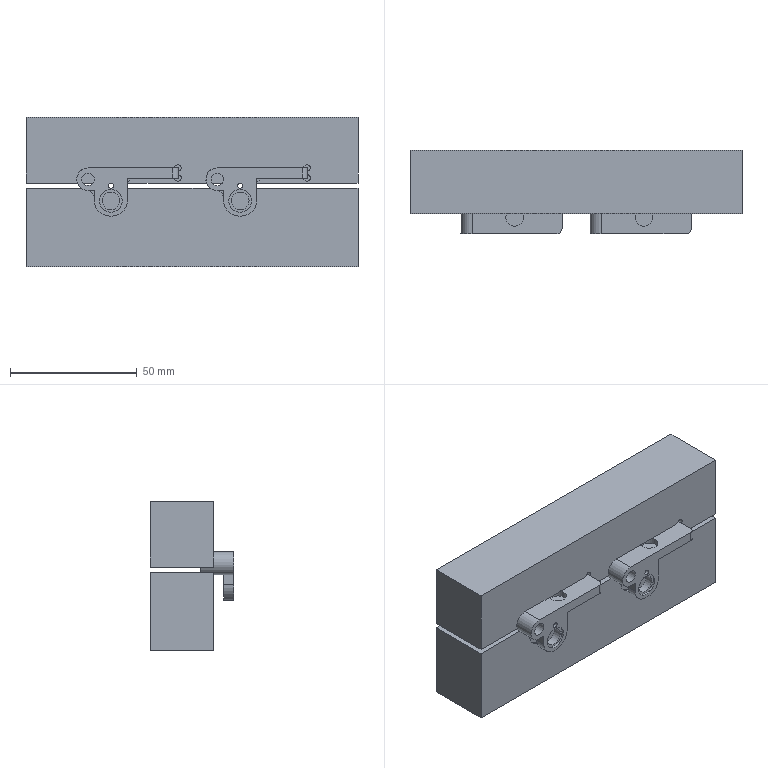CAM job | NX | 3+2 milling, drilling | part box 131 x 33 x 59 mm
Tools:
number,name,description,diameter,corner_radius,flute_length,length,flutes
3,D3,平底铣刀-粗,3.0,0.0,20.0,75.0,2
4,D4,平底铣刀-粗,4.0,0.0,25.0,75.0,2
8,D8,平底铣刀-粗,8.0,0.0,30.0,75.0,2
9,D10,平底铣刀-粗,10.0,0.0,35.0,75.0,2
17,D2-J,平底铣刀-精,2.0,0.0,50.0,75.0,2
11,D4-J,平底铣刀-精,4.0,0.0,50.0,75.0,2
7,D6-J,平底铣刀-精,6.0,0.0,25.0,75.0,2
10,D10-J,平底铣刀-精,10.0,0.0,35.0,75.0,2
1,D80R0.8飞刀,圆鼻刀-粗,80.0,0.8,50.0,75.0,2
2,D6倒角刀,倒角刀,6.0,0.0,3.0,25.0,2
19,M2.5X0.45,丝锥,2.05,0.0,35.0,50.0,2
20,D5铰刀,Drilling Tool,5.0,0.0,75.0,100.0,6
17,ZT2.1,钻头,2.1,0.0,35.0,50.0,2
18,ZT4.9,Drilling Tool,4.9,0.0,35.0,50.0,2
16,ZT6.9,Drilling Tool,6.9,0.0,35.0,50.0,2
Operations:
program,operation,operation_type,tool,method,geometry_group,spindle_rpm,surface_speed,feed_per_tooth,feed_cut,feed_plunge,cut_length_mm,path_length_mm,cut_time_min,machine_time_min
E,BOTTOMWALL-LAYERROUGH-MED_COPY,VolumeBased25DMillingOperation,D3,LAYERROUGH-DEPTHK-STEPG,W-E,8000.0,75.398,0.125,2000.0,100.0,7701.758,7880.728,3.851,3.869
E,ZLEVEL-SMOOTH-CORNERD2-REF6_COPY_2,ZLevelMilling,D2-J,LAYERFINISH-DEPTHK-STEPG,W-E,8000.0,50.264,0.05,800.0,100.0,1220.015,1495.166,1.525,1.552
E,BOTTOMWALL-FINISHFLOOR-MED_COPY_2,VolumeBased25DMillingOperation,D2-J,FINISH-STEPDEPTH-OFF,W-E,7000.0,175.0,0.0536,1500.0,100.0,533.255,631.029,0.3555,0.3653
E,BOTTOMWALL-FINISHFLOOR-MED_COPY_2_COPY,VolumeBased25DMillingOperation,D2-J,FINISH-STEPDEPTH-OFF,W-E,7000.0,175.0,0.0536,1500.0,100.0,244.848,349.977,0.1632,0.1737
E,C0.3CLOSEDCONTOUR-CHAMFER6X45L_COPY_1,PlanarMilling,D6倒角刀,WALLCLIMB_CHAMFER-DEPTH0-STEPG,W-E,7000.0,131.0,0.1071,1500.0,100.0,242.143,477.193,0.1614,0.1849
E,BOTTOMWALL-FINISHSIDE-MED_COPY_1,VolumeBased25DMillingOperation,D2-J,SIDEFINISH-DEPTHK-STEPG,W-E,8000.0,50.264,0.0375,600.0,100.0,148.402,265.878,0.2473,0.2591
E,BOTTOMWALL-FINISHSIDE-MED_COPY_2,VolumeBased25DMillingOperation,D2-J,SIDEFINISH-DEPTHK-STEPG,W-E,8000.0,50.264,0.0375,600.0,100.0,719.738,928.916,1.2,1.22
D,BOTTOMWALL-FINISHSIDE-MED_COPY,VolumeBased25DMillingOperation,D4,SIDEFINISH-DEPTHK-STEPG,W-D,8000.0,100.531,0.125,2000.0,100.0,1801.594,1936.513,0.9008,0.9143
D,BOTTOMWALL-FINISHFLOOR-MED_COPY_1,VolumeBased25DMillingOperation,D4-J,FINISH-STEPDEPTH-OFF,W-D,7000.0,175.0,0.0536,1500.0,100.0,196.489,244.289,0.131,0.1358
D,BOTTOMWALL-FINISHSIDE-MED-SELFLOOR_COPY_1,VolumeBased25DMillingOperation,D4-J,SIDEFINISH-DEPTHK-STEPG,W-D,8000.0,100.528,0.05,800.0,100.0,43.658,96.602,0.0546,0.0599
D,BOTTOMWALL-FINISHSIDE-MED-SELFLOOR_COPY,VolumeBased25DMillingOperation,D4-J,SIDEFINISH-DEPTHK-STEPG,W-D,8000.0,100.528,0.05,800.0,100.0,154.98,232.252,0.1937,0.2015
D,ZLEVEL-SMOOTH-CORNERD2-REF6_COPY_1,ZLevelMilling,D2-J,LAYERFINISH-DEPTHK-STEPG,W-D,8000.0,50.264,0.05,800.0,100.0,411.487,567.042,0.5144,0.5299
C,BOTTOMWALL-HELIXROUGH-SMALL_COPY_1,VolumeBased25DMillingOperation,D4,LAYERROUGH-DEPTHK-STEPG,W-C,8000.0,100.531,0.0375,600.0,100.0,107.628,208.468,0.1794,0.1895
C,C0.3CLOSEDCONTOUR-CHAMFER6X45L_COPY,PlanarMilling,D6倒角刀,WALLCLIMB_CHAMFER-DEPTH0-STEPG,W-C,7000.0,131.0,0.1071,1500.0,100.0,30.826,126.826,0.0206,0.0302
C,BOTTOMWALL-HELIXFINISH-SMALL_COPY_1,VolumeBased25DMillingOperation,D4-J,HELIXFINISH-DEPTHK-STEPG,W-C,8000.0,100.531,0.0312,500.0,100.0,39.572,140.572,0.0791,0.0892
B,DYNAMICROUGHD10_COPY_1,CavityMilling,D10,DYNAMICROUGH-DEPTHK-STEPK,W-B,8000.0,251.32,0.25,4000.0,100.0,4082.757,4178.557,1.021,1.03
B,BOTTOMWALL-FINISHFLOOR-MED_COPY,VolumeBased25DMillingOperation,D10-J,FINISH-STEPDEPTH-OFF,W-B,7000.0,175.0,0.0536,1500.0,100.0,464.965,513.828,0.31,0.3149
B,BOTTOMWALL-HELIXROUGH-SMALL_COPY,VolumeBased25DMillingOperation,D4,LAYERROUGH-DEPTHK-STEPG,W-B,8000.0,100.528,0.125,2000.0,100.0,183.783,432.172,0.0919,0.1167
B,DRILLCHAMFER-DJ10_1,Operation,D6倒角刀,METHOD,W-B,8000.0,150.796,0.0625,1000.0,0.0,11.6,177.288,0.0116,0.0282
B,DRILLCHAMFER_2,Operation,D6倒角刀,METHOD,W-B,8000.0,150.796,0.0312,500.0,0.0,8.95,171.988,0.0179,0.0342
B,PLANARDEBURR6X45L_COPY_1,SurfaceContour,D6倒角刀,WALLCLIMB_CHAMFER-DEPTH0-STEPG,W-B,6500.0,122.519,0.1154,1500.0,100.0,347.241,772.849,0.2315,0.2741
B,BOTTOMWALL-HELIXFINISH-SMALL_COPY,VolumeBased25DMillingOperation,D4-J,HELIXFINISH-DEPTHK-STEPG,W-B,8000.0,100.531,0.0375,600.0,100.0,85.16,333.305,0.1419,0.1667
B,ZLEVEL-FINISHRECIPCLIMB_COPY_COPY,ZLevelMilling,D4-J,ZLEVELWALLCLIMB-DEPTHK-STEPG,W-B,7000.0,131.947,0.25,3500.0,100.0,2472.834,2576.49,0.7065,0.7169
A,TOPFACE,FaceMilling,D80R0.8飞刀,SIDEFINISH-DEPTHK-STEPG,W-A,4500.0,1385.0,0.1667,1500.0,100.0,185.0,281.0,0.1233,0.1329
A,DYNAMICROUGHD10_COPY,CavityMilling,D8,DYNAMICROUGH-DEPTHK-STEPK,W-A,8000.0,251.32,0.25,4000.0,100.0,3620.391,4719.744,0.9051,1.015
A,SPOT-DEPTH0.8,Operation,D6倒角刀,NONE,W-A,8000.0,150.796,0.0312,500.0,90.0,10.8,200.417,0.0216,0.0406
A,THRUHOLE-M2.5TAPDRILL,Operation,ZT2.1,NONE,W-A,3000.0,19.321,0.0333,200.0,90.0,42.0,236.01,0.21,0.2294
A,THRUHOLE-FINE6.0PREDRILL,Operation,ZT4.9,NONE,W-A,2500.0,38.484,0.05,250.0,90.0,36.829,225.668,0.1473,0.1662
A,3STEPHOLE-G83DRILL,Operation,ZT6.9,NONE,W-A,1500.0,32.987,0.04,120.0,90.0,36.0,224.01,0.3,0.3188
A,3STEPHOLE-MILLROUGH1_1,CylinderMilling,D4,NONE,W-A,8000.0,100.531,0.075,1200.0,100.0,269.468,523.668,0.2246,0.25
A,3STEPHOLE-MILLROUGH2_1,CylinderMilling,D4,NONE,W-A,8000.0,100.531,0.075,1200.0,100.0,799.116,1076.716,0.6659,0.6937
A,3STEPHOLE-MILLFINISH1_1,CylinderMilling,D4-J,FINISH-STEPDEPTH-OFF,W-A,8000.0,100.531,0.0312,500.0,100.0,55.602,307.202,0.1112,0.1364
A,ZLEVEL-SMOOTH-CORNERD2-REF6_COPY,ZLevelMilling,D4-J,LAYERFINISH-DEPTHK-STEPG,W-A,8000.0,50.266,0.125,2000.0,100.0,2431.683,2992.25,1.216,1.272
A,DRILLCHAMFER_1,Operation,D6倒角刀,METHOD,W-A,8000.0,150.796,0.0312,500.0,0.0,8.95,171.988,0.0179,0.0342
A,MILLCHAMFER_1,PlanarMilling,D6倒角刀,METHOD,W-A,8000.0,150.796,0.0312,500.0,100.0,36.963,288.394,0.0739,0.0991
A,PLANARDEBURR6X45L_COPY,SurfaceContour,D6倒角刀,WALLCLIMB_CHAMFER-DEPTH0-STEPG,W-A,6500.0,122.519,0.1154,1500.0,100.0,347.277,759.67,0.2315,0.2728
A,3STEPHOLE-MILLFINISH2_1,CylinderMilling,D4-J,FINISH-STEPDEPTH-OFF,W-A,8000.0,100.531,0.025,400.0,100.0,82.795,360.395,0.207,0.2347
A,REAM,Operation,D5铰刀,METHOD,W-A,500.0,7.854,0.0167,50.0,0.0,30.0,212.01,0.6,0.6182
A,THRUHOLE-TAPM2.5,Operation,M2.5X0.45,METHOD,W-A,1000.0,6.44,0.0002,0.45,90.0,34.0,220.01,75.556,75.574
A,ZLEVEL-FINISHRECIPCLIMB_COPY,ZLevelMilling,D6-J,ZLEVELWALLCLIMB-DEPTHK-STEPG,W-A,7000.0,131.947,0.25,3500.0,100.0,2468.735,2566.729,0.7054,0.7152
A,PROFILESEMIFIN_2,VolumeBased25DMillingOperation,D6-J,METHOD,W-A,9000.0,169.646,0.0667,1200.0,100.0,520.774,1053.332,0.434,0.4872